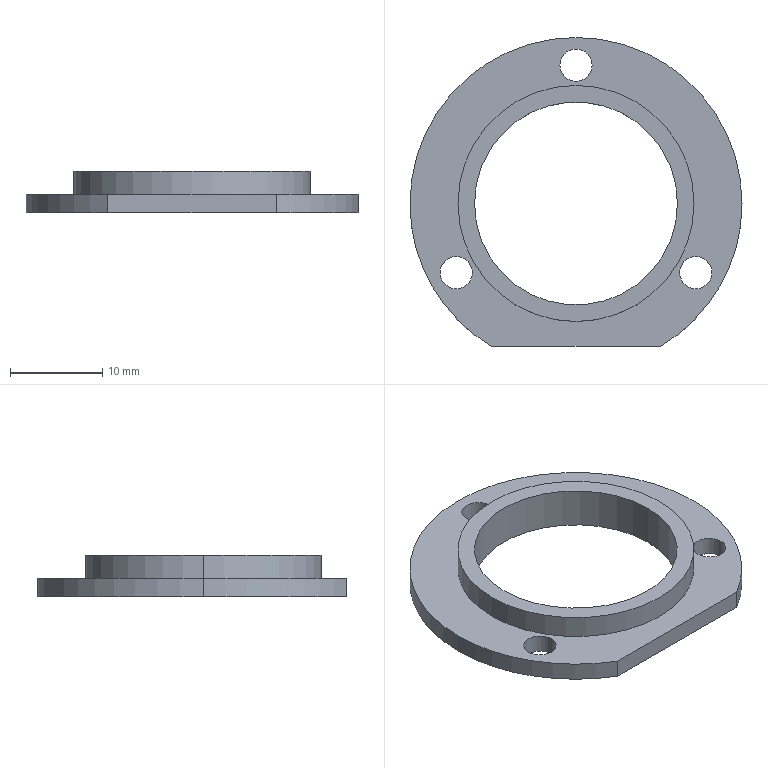Part | SolidWorks | features ICE 3, Extrusion 1 | 1 solid | 17 faces | box 36 x 33.5 x 4.5 mm | volume 1492 mm3 | cylinder 13 | plane 4 | commonest cylinder face diameters 3.5 x6 36 x3 22 x2 25.6 x2
STEP:
#1=CARTESIAN_POINT('',(-14.74,-7.5,2.));
#2=VERTEX_POINT('',#1);
#3=CARTESIAN_POINT('',(-11.24,-7.5,2.));
#4=VERTEX_POINT('',#3);
#5=CARTESIAN_POINT('',(-12.99,-7.5,2.));
#6=DIRECTION('',(0.,0.,1.));
#7=DIRECTION('',(1.,0.,0.));
#8=AXIS2_PLACEMENT_3D('',#5,#6,#7);
#9=CIRCLE('',#8,1.75);
#10=EDGE_CURVE('',#2,#4,#9,.T.);
#11=ORIENTED_EDGE('',*,*,#10,.T.);
#12=CARTESIAN_POINT('',(-11.24,-7.5,0.));
#13=VERTEX_POINT('',#12);
#14=CARTESIAN_POINT('',(-11.24,-7.5,4.5));
#15=DIRECTION('',(0.,0.,-1.));
#16=VECTOR('',#15,1000.);
#17=LINE('',#14,#16);
#18=EDGE_CURVE('',#4,#13,#17,.T.);
#19=ORIENTED_EDGE('',*,*,#18,.T.);
#20=CARTESIAN_POINT('',(-14.74,-7.5,0.));
#21=VERTEX_POINT('',#20);
#22=CARTESIAN_POINT('',(-12.99,-7.5,0.));
#23=DIRECTION('',(0.,0.,-1.));
#24=DIRECTION('',(-1.,0.,0.));
#25=AXIS2_PLACEMENT_3D('',#22,#23,#24);
#26=CIRCLE('',#25,1.75);
#27=EDGE_CURVE('',#13,#21,#26,.T.);
#28=ORIENTED_EDGE('',*,*,#27,.T.);
#29=CARTESIAN_POINT('',(-14.74,-7.5,4.5));
#30=DIRECTION('',(0.,0.,-1.));
#31=VECTOR('',#30,1000.);
#32=LINE('',#29,#31);
#33=EDGE_CURVE('',#2,#21,#32,.T.);
#34=ORIENTED_EDGE('',*,*,#33,.F.);
#35=EDGE_LOOP('',(#11,#19,#28,#34));
#36=FACE_OUTER_BOUND('',#35,.T.);
#37=CARTESIAN_POINT('',(-12.99,-7.5,4.5));
#38=DIRECTION('',(0.,0.,-1.));
#39=DIRECTION('',(-1.,0.,0.));
#40=AXIS2_PLACEMENT_3D('',#37,#38,#39);
#41=CYLINDRICAL_SURFACE('',#40,1.75);
#42=ADVANCED_FACE('',(#36),#41,.F.);
#43=CARTESIAN_POINT('',(11.24,-7.5,2.));
#44=VERTEX_POINT('',#43);
#45=CARTESIAN_POINT('',(14.74,-7.5,2.));
#46=VERTEX_POINT('',#45);
#47=CARTESIAN_POINT('',(12.99,-7.5,2.));
#48=DIRECTION('',(0.,0.,1.));
#49=DIRECTION('',(1.,0.,0.));
#50=AXIS2_PLACEMENT_3D('',#47,#48,#49);
#51=CIRCLE('',#50,1.75);
#52=EDGE_CURVE('',#44,#46,#51,.T.);
#53=ORIENTED_EDGE('',*,*,#52,.T.);
#54=CARTESIAN_POINT('',(14.74,-7.5,0.));
#55=VERTEX_POINT('',#54);
#56=CARTESIAN_POINT('',(14.74,-7.5,4.5));
#57=DIRECTION('',(0.,0.,-1.));
#58=VECTOR('',#57,1000.);
#59=LINE('',#56,#58);
#60=EDGE_CURVE('',#46,#55,#59,.T.);
#61=ORIENTED_EDGE('',*,*,#60,.T.);
#62=CARTESIAN_POINT('',(11.24,-7.5,0.));
#63=VERTEX_POINT('',#62);
#64=CARTESIAN_POINT('',(12.99,-7.5,0.));
#65=DIRECTION('',(0.,0.,-1.));
#66=DIRECTION('',(-1.,0.,0.));
#67=AXIS2_PLACEMENT_3D('',#64,#65,#66);
#68=CIRCLE('',#67,1.75);
#69=EDGE_CURVE('',#55,#63,#68,.T.);
#70=ORIENTED_EDGE('',*,*,#69,.T.);
#71=CARTESIAN_POINT('',(11.24,-7.5,4.5));
#72=DIRECTION('',(0.,0.,-1.));
#73=VECTOR('',#72,1000.);
#74=LINE('',#71,#73);
#75=EDGE_CURVE('',#44,#63,#74,.T.);
#76=ORIENTED_EDGE('',*,*,#75,.F.);
#77=EDGE_LOOP('',(#53,#61,#70,#76));
#78=FACE_OUTER_BOUND('',#77,.T.);
#79=CARTESIAN_POINT('',(12.99,-7.5,4.5));
#80=DIRECTION('',(0.,0.,-1.));
#81=DIRECTION('',(-1.,0.,0.));
#82=AXIS2_PLACEMENT_3D('',#79,#80,#81);
#83=CYLINDRICAL_SURFACE('',#82,1.75);
#84=ADVANCED_FACE('',(#78),#83,.F.);
#85=CARTESIAN_POINT('',(-1.75,15.,2.));
#86=VERTEX_POINT('',#85);
#87=CARTESIAN_POINT('',(1.75,15.,2.));
#88=VERTEX_POINT('',#87);
#89=CARTESIAN_POINT('',(0.,15.,2.));
#90=DIRECTION('',(0.,0.,1.));
#91=DIRECTION('',(1.,0.,0.));
#92=AXIS2_PLACEMENT_3D('',#89,#90,#91);
#93=CIRCLE('',#92,1.75);
#94=EDGE_CURVE('',#86,#88,#93,.T.);
#95=ORIENTED_EDGE('',*,*,#94,.T.);
#96=CARTESIAN_POINT('',(1.75,15.,0.));
#97=VERTEX_POINT('',#96);
#98=CARTESIAN_POINT('',(1.75,15.,4.5));
#99=DIRECTION('',(0.,0.,-1.));
#100=VECTOR('',#99,1000.);
#101=LINE('',#98,#100);
#102=EDGE_CURVE('',#88,#97,#101,.T.);
#103=ORIENTED_EDGE('',*,*,#102,.T.);
#104=CARTESIAN_POINT('',(-1.75,15.,0.));
#105=VERTEX_POINT('',#104);
#106=CARTESIAN_POINT('',(0.,15.,0.));
#107=DIRECTION('',(0.,0.,-1.));
#108=DIRECTION('',(-1.,0.,0.));
#109=AXIS2_PLACEMENT_3D('',#106,#107,#108);
#110=CIRCLE('',#109,1.75);
#111=EDGE_CURVE('',#97,#105,#110,.T.);
#112=ORIENTED_EDGE('',*,*,#111,.T.);
#113=CARTESIAN_POINT('',(-1.75,15.,4.5));
#114=DIRECTION('',(0.,0.,-1.));
#115=VECTOR('',#114,1000.);
#116=LINE('',#113,#115);
#117=EDGE_CURVE('',#86,#105,#116,.T.);
#118=ORIENTED_EDGE('',*,*,#117,.F.);
#119=EDGE_LOOP('',(#95,#103,#112,#118));
#120=FACE_OUTER_BOUND('',#119,.T.);
#121=CARTESIAN_POINT('',(0.,15.,4.5));
#122=DIRECTION('',(0.,0.,-1.));
#123=DIRECTION('',(-1.,0.,0.));
#124=AXIS2_PLACEMENT_3D('',#121,#122,#123);
#125=CYLINDRICAL_SURFACE('',#124,1.75);
#126=ADVANCED_FACE('',(#120),#125,.F.);
#127=CARTESIAN_POINT('',(12.8,0.,2.));
#128=VERTEX_POINT('',#127);
#129=CARTESIAN_POINT('',(-12.8,0.,2.));
#130=VERTEX_POINT('',#129);
#131=CARTESIAN_POINT('',(0.,0.,2.));
#132=DIRECTION('',(0.,0.,1.));
#133=DIRECTION('',(1.,0.,0.));
#134=AXIS2_PLACEMENT_3D('',#131,#132,#133);
#135=CIRCLE('',#134,12.8);
#136=EDGE_CURVE('',#128,#130,#135,.T.);
#137=ORIENTED_EDGE('',*,*,#136,.T.);
#138=CARTESIAN_POINT('',(-12.8,0.,4.5));
#139=VERTEX_POINT('',#138);
#140=CARTESIAN_POINT('',(-12.8,0.,2.));
#141=DIRECTION('',(0.,0.,1.));
#142=VECTOR('',#141,1000.);
#143=LINE('',#140,#142);
#144=EDGE_CURVE('',#130,#139,#143,.T.);
#145=ORIENTED_EDGE('',*,*,#144,.T.);
#146=CARTESIAN_POINT('',(12.8,0.,4.5));
#147=VERTEX_POINT('',#146);
#148=CARTESIAN_POINT('',(0.,0.,4.5));
#149=DIRECTION('',(0.,0.,1.));
#150=DIRECTION('',(1.,0.,0.));
#151=AXIS2_PLACEMENT_3D('',#148,#149,#150);
#152=CIRCLE('',#151,12.8);
#153=EDGE_CURVE('',#147,#139,#152,.T.);
#154=ORIENTED_EDGE('',*,*,#153,.F.);
#155=CARTESIAN_POINT('',(12.8,0.,2.));
#156=DIRECTION('',(0.,0.,1.));
#157=VECTOR('',#156,1000.);
#158=LINE('',#155,#157);
#159=EDGE_CURVE('',#128,#147,#158,.T.);
#160=ORIENTED_EDGE('',*,*,#159,.F.);
#161=EDGE_LOOP('',(#137,#145,#154,#160));
#162=FACE_OUTER_BOUND('',#161,.T.);
#163=CARTESIAN_POINT('',(0.,0.,2.));
#164=DIRECTION('',(0.,0.,1.));
#165=DIRECTION('',(1.,0.,0.));
#166=AXIS2_PLACEMENT_3D('',#163,#164,#165);
#167=CYLINDRICAL_SURFACE('',#166,12.8);
#168=ADVANCED_FACE('',(#162),#167,.T.);
#169=CARTESIAN_POINT('',(-11.,0.,4.5));
#170=VERTEX_POINT('',#169);
#171=CARTESIAN_POINT('',(11.,0.,4.5));
#172=VERTEX_POINT('',#171);
#173=CARTESIAN_POINT('',(0.,0.,4.5));
#174=DIRECTION('',(0.,0.,1.));
#175=DIRECTION('',(1.,0.,0.));
#176=AXIS2_PLACEMENT_3D('',#173,#174,#175);
#177=CIRCLE('',#176,11.);
#178=EDGE_CURVE('',#170,#172,#177,.T.);
#179=ORIENTED_EDGE('',*,*,#178,.T.);
#180=CARTESIAN_POINT('',(11.,0.,0.));
#181=VERTEX_POINT('',#180);
#182=CARTESIAN_POINT('',(11.,0.,4.5));
#183=DIRECTION('',(0.,0.,-1.));
#184=VECTOR('',#183,1000.);
#185=LINE('',#182,#184);
#186=EDGE_CURVE('',#172,#181,#185,.T.);
#187=ORIENTED_EDGE('',*,*,#186,.T.);
#188=CARTESIAN_POINT('',(-11.,0.,0.));
#189=VERTEX_POINT('',#188);
#190=CARTESIAN_POINT('',(0.,0.,0.));
#191=DIRECTION('',(0.,0.,1.));
#192=DIRECTION('',(1.,0.,0.));
#193=AXIS2_PLACEMENT_3D('',#190,#191,#192);
#194=CIRCLE('',#193,11.);
#195=EDGE_CURVE('',#189,#181,#194,.T.);
#196=ORIENTED_EDGE('',*,*,#195,.F.);
#197=CARTESIAN_POINT('',(-11.,0.,4.5));
#198=DIRECTION('',(0.,0.,-1.));
#199=VECTOR('',#198,1000.);
#200=LINE('',#197,#199);
#201=EDGE_CURVE('',#170,#189,#200,.T.);
#202=ORIENTED_EDGE('',*,*,#201,.F.);
#203=EDGE_LOOP('',(#179,#187,#196,#202));
#204=FACE_OUTER_BOUND('',#203,.T.);
#205=CARTESIAN_POINT('',(0.,0.,4.5));
#206=DIRECTION('',(0.,0.,-1.));
#207=DIRECTION('',(-1.,0.,0.));
#208=AXIS2_PLACEMENT_3D('',#205,#206,#207);
#209=CYLINDRICAL_SURFACE('',#208,11.);
#210=ADVANCED_FACE('',(#204),#209,.F.);
#211=CARTESIAN_POINT('',(18.,0.,2.));
#212=VERTEX_POINT('',#211);
#213=CARTESIAN_POINT('',(-18.,0.,2.));
#214=VERTEX_POINT('',#213);
#215=CARTESIAN_POINT('',(0.,0.,2.));
#216=DIRECTION('',(0.,0.,1.));
#217=DIRECTION('',(1.,0.,0.));
#218=AXIS2_PLACEMENT_3D('',#215,#216,#217);
#219=CIRCLE('',#218,18.);
#220=EDGE_CURVE('',#212,#214,#219,.T.);
#221=ORIENTED_EDGE('',*,*,#220,.F.);
#222=CARTESIAN_POINT('',(18.,0.,0.));
#223=VERTEX_POINT('',#222);
#224=CARTESIAN_POINT('',(18.,0.,4.5));
#225=DIRECTION('',(0.,0.,-1.));
#226=VECTOR('',#225,1000.);
#227=LINE('',#224,#226);
#228=EDGE_CURVE('',#212,#223,#227,.T.);
#229=ORIENTED_EDGE('',*,*,#228,.T.);
#230=CARTESIAN_POINT('',(-18.,0.,0.));
#231=VERTEX_POINT('',#230);
#232=CARTESIAN_POINT('',(0.,0.,0.));
#233=DIRECTION('',(0.,0.,1.));
#234=DIRECTION('',(1.,0.,0.));
#235=AXIS2_PLACEMENT_3D('',#232,#233,#234);
#236=CIRCLE('',#235,18.);
#237=EDGE_CURVE('',#223,#231,#236,.T.);
#238=ORIENTED_EDGE('',*,*,#237,.T.);
#239=CARTESIAN_POINT('',(-18.,0.,4.5));
#240=DIRECTION('',(0.,0.,-1.));
#241=VECTOR('',#240,1000.);
#242=LINE('',#239,#241);
#243=EDGE_CURVE('',#214,#231,#242,.T.);
#244=ORIENTED_EDGE('',*,*,#243,.F.);
#245=EDGE_LOOP('',(#221,#229,#238,#244));
#246=FACE_OUTER_BOUND('',#245,.T.);
#247=CARTESIAN_POINT('',(0.,0.,4.5));
#248=DIRECTION('',(0.,0.,-1.));
#249=DIRECTION('',(-1.,0.,0.));
#250=AXIS2_PLACEMENT_3D('',#247,#248,#249);
#251=CYLINDRICAL_SURFACE('',#250,18.);
#252=ADVANCED_FACE('',(#246),#251,.T.);
#253=CARTESIAN_POINT('',(-9.152,-15.5,2.));
#254=VERTEX_POINT('',#253);
#255=CARTESIAN_POINT('',(0.,0.,2.));
#256=DIRECTION('',(0.,0.,1.));
#257=DIRECTION('',(1.,0.,0.));
#258=AXIS2_PLACEMENT_3D('',#255,#256,#257);
#259=CIRCLE('',#258,18.);
#260=EDGE_CURVE('',#214,#254,#259,.T.);
#261=ORIENTED_EDGE('',*,*,#260,.F.);
#262=ORIENTED_EDGE('',*,*,#243,.T.);
#263=CARTESIAN_POINT('',(-9.152,-15.5,0.));
#264=VERTEX_POINT('',#263);
#265=CARTESIAN_POINT('',(0.,0.,0.));
#266=DIRECTION('',(0.,0.,1.));
#267=DIRECTION('',(1.,0.,0.));
#268=AXIS2_PLACEMENT_3D('',#265,#266,#267);
#269=CIRCLE('',#268,18.);
#270=EDGE_CURVE('',#231,#264,#269,.T.);
#271=ORIENTED_EDGE('',*,*,#270,.T.);
#272=CARTESIAN_POINT('',(-9.152,-15.5,4.5));
#273=DIRECTION('',(0.,0.,1.));
#274=VECTOR('',#273,1000.);
#275=LINE('',#272,#274);
#276=EDGE_CURVE('',#264,#254,#275,.T.);
#277=ORIENTED_EDGE('',*,*,#276,.T.);
#278=EDGE_LOOP('',(#261,#262,#271,#277));
#279=FACE_OUTER_BOUND('',#278,.T.);
#280=CARTESIAN_POINT('',(0.,0.,4.5));
#281=DIRECTION('',(0.,0.,-1.));
#282=DIRECTION('',(-1.,0.,0.));
#283=AXIS2_PLACEMENT_3D('',#280,#281,#282);
#284=CYLINDRICAL_SURFACE('',#283,18.);
#285=ADVANCED_FACE('',(#279),#284,.T.);
#286=ORIENTED_EDGE('',*,*,#178,.F.);
#287=CARTESIAN_POINT('',(0.,0.,4.5));
#288=DIRECTION('',(0.,0.,1.));
#289=DIRECTION('',(1.,0.,0.));
#290=AXIS2_PLACEMENT_3D('',#287,#288,#289);
#291=CIRCLE('',#290,11.);
#292=EDGE_CURVE('',#172,#170,#291,.T.);
#293=ORIENTED_EDGE('',*,*,#292,.F.);
#294=EDGE_LOOP('',(#286,#293));
#295=FACE_BOUND('',#294,.T.);
#296=ORIENTED_EDGE('',*,*,#153,.T.);
#297=CARTESIAN_POINT('',(0.,0.,4.5));
#298=DIRECTION('',(0.,0.,1.));
#299=DIRECTION('',(1.,0.,0.));
#300=AXIS2_PLACEMENT_3D('',#297,#298,#299);
#301=CIRCLE('',#300,12.8);
#302=EDGE_CURVE('',#139,#147,#301,.T.);
#303=ORIENTED_EDGE('',*,*,#302,.T.);
#304=EDGE_LOOP('',(#296,#303));
#305=FACE_OUTER_BOUND('',#304,.T.);
#306=CARTESIAN_POINT('',(0.,0.,4.5));
#307=DIRECTION('',(0.,0.,1.));
#308=DIRECTION('',(1.,0.,0.));
#309=AXIS2_PLACEMENT_3D('',#306,#307,#308);
#310=PLANE('',#309);
#311=ADVANCED_FACE('',(#295,#305),#310,.T.);
#312=ORIENTED_EDGE('',*,*,#228,.F.);
#313=CARTESIAN_POINT('',(9.152,-15.5,2.));
#314=VERTEX_POINT('',#313);
#315=CARTESIAN_POINT('',(0.,0.,2.));
#316=DIRECTION('',(0.,0.,1.));
#317=DIRECTION('',(1.,0.,0.));
#318=AXIS2_PLACEMENT_3D('',#315,#316,#317);
#319=CIRCLE('',#318,18.);
#320=EDGE_CURVE('',#314,#212,#319,.T.);
#321=ORIENTED_EDGE('',*,*,#320,.F.);
#322=CARTESIAN_POINT('',(9.152,-15.5,0.));
#323=VERTEX_POINT('',#322);
#324=CARTESIAN_POINT('',(9.152,-15.5,4.5));
#325=DIRECTION('',(0.,0.,-1.));
#326=VECTOR('',#325,1000.);
#327=LINE('',#324,#326);
#328=EDGE_CURVE('',#314,#323,#327,.T.);
#329=ORIENTED_EDGE('',*,*,#328,.T.);
#330=CARTESIAN_POINT('',(0.,0.,0.));
#331=DIRECTION('',(0.,0.,1.));
#332=DIRECTION('',(1.,0.,0.));
#333=AXIS2_PLACEMENT_3D('',#330,#331,#332);
#334=CIRCLE('',#333,18.);
#335=EDGE_CURVE('',#323,#223,#334,.T.);
#336=ORIENTED_EDGE('',*,*,#335,.T.);
#337=EDGE_LOOP('',(#312,#321,#329,#336));
#338=FACE_OUTER_BOUND('',#337,.T.);
#339=CARTESIAN_POINT('',(0.,0.,4.5));
#340=DIRECTION('',(0.,0.,-1.));
#341=DIRECTION('',(-1.,0.,0.));
#342=AXIS2_PLACEMENT_3D('',#339,#340,#341);
#343=CYLINDRICAL_SURFACE('',#342,18.);
#344=ADVANCED_FACE('',(#338),#343,.T.);
#345=CARTESIAN_POINT('',(-12.99,-7.5,0.));
#346=DIRECTION('',(0.,0.,-1.));
#347=DIRECTION('',(-1.,0.,0.));
#348=AXIS2_PLACEMENT_3D('',#345,#346,#347);
#349=CIRCLE('',#348,1.75);
#350=EDGE_CURVE('',#21,#13,#349,.T.);
#351=ORIENTED_EDGE('',*,*,#350,.F.);
#352=ORIENTED_EDGE('',*,*,#27,.F.);
#353=EDGE_LOOP('',(#351,#352));
#354=FACE_BOUND('',#353,.T.);
#355=CARTESIAN_POINT('',(12.99,-7.5,0.));
#356=DIRECTION('',(0.,0.,-1.));
#357=DIRECTION('',(-1.,0.,0.));
#358=AXIS2_PLACEMENT_3D('',#355,#356,#357);
#359=CIRCLE('',#358,1.75);
#360=EDGE_CURVE('',#63,#55,#359,.T.);
#361=ORIENTED_EDGE('',*,*,#360,.F.);
#362=ORIENTED_EDGE('',*,*,#69,.F.);
#363=EDGE_LOOP('',(#361,#362));
#364=FACE_BOUND('',#363,.T.);
#365=CARTESIAN_POINT('',(0.,15.,0.));
#366=DIRECTION('',(0.,0.,-1.));
#367=DIRECTION('',(-1.,0.,0.));
#368=AXIS2_PLACEMENT_3D('',#365,#366,#367);
#369=CIRCLE('',#368,1.75);
#370=EDGE_CURVE('',#105,#97,#369,.T.);
#371=ORIENTED_EDGE('',*,*,#370,.F.);
#372=ORIENTED_EDGE('',*,*,#111,.F.);
#373=EDGE_LOOP('',(#371,#372));
#374=FACE_BOUND('',#373,.T.);
#375=ORIENTED_EDGE('',*,*,#335,.F.);
#376=CARTESIAN_POINT('',(-24.788,-15.5,0.));
#377=DIRECTION('',(-1.,0.,0.));
#378=VECTOR('',#377,1000.);
#379=LINE('',#376,#378);
#380=EDGE_CURVE('',#323,#264,#379,.T.);
#381=ORIENTED_EDGE('',*,*,#380,.T.);
#382=ORIENTED_EDGE('',*,*,#270,.F.);
#383=ORIENTED_EDGE('',*,*,#237,.F.);
#384=EDGE_LOOP('',(#375,#381,#382,#383));
#385=FACE_OUTER_BOUND('',#384,.T.);
#386=ORIENTED_EDGE('',*,*,#195,.T.);
#387=CARTESIAN_POINT('',(0.,0.,0.));
#388=DIRECTION('',(0.,0.,1.));
#389=DIRECTION('',(1.,0.,0.));
#390=AXIS2_PLACEMENT_3D('',#387,#388,#389);
#391=CIRCLE('',#390,11.);
#392=EDGE_CURVE('',#181,#189,#391,.T.);
#393=ORIENTED_EDGE('',*,*,#392,.T.);
#394=EDGE_LOOP('',(#386,#393));
#395=FACE_BOUND('',#394,.T.);
#396=CARTESIAN_POINT('',(0.,0.,0.));
#397=DIRECTION('',(0.,0.,1.));
#398=DIRECTION('',(1.,0.,0.));
#399=AXIS2_PLACEMENT_3D('',#396,#397,#398);
#400=PLANE('',#399);
#401=ADVANCED_FACE('',(#354,#364,#374,#385,#395),#400,.F.);
#402=ORIENTED_EDGE('',*,*,#186,.F.);
#403=ORIENTED_EDGE('',*,*,#292,.T.);
#404=ORIENTED_EDGE('',*,*,#201,.T.);
#405=ORIENTED_EDGE('',*,*,#392,.F.);
#406=EDGE_LOOP('',(#402,#403,#404,#405));
#407=FACE_OUTER_BOUND('',#406,.T.);
#408=CARTESIAN_POINT('',(0.,0.,4.5));
#409=DIRECTION('',(0.,0.,-1.));
#410=DIRECTION('',(-1.,0.,0.));
#411=AXIS2_PLACEMENT_3D('',#408,#409,#410);
#412=CYLINDRICAL_SURFACE('',#411,11.);
#413=ADVANCED_FACE('',(#407),#412,.F.);
#414=ORIENTED_EDGE('',*,*,#10,.F.);
#415=CARTESIAN_POINT('',(-12.99,-7.5,2.));
#416=DIRECTION('',(0.,0.,1.));
#417=DIRECTION('',(1.,0.,0.));
#418=AXIS2_PLACEMENT_3D('',#415,#416,#417);
#419=CIRCLE('',#418,1.75);
#420=EDGE_CURVE('',#4,#2,#419,.T.);
#421=ORIENTED_EDGE('',*,*,#420,.F.);
#422=EDGE_LOOP('',(#414,#421));
#423=FACE_BOUND('',#422,.T.);
#424=ORIENTED_EDGE('',*,*,#52,.F.);
#425=CARTESIAN_POINT('',(12.99,-7.5,2.));
#426=DIRECTION('',(0.,0.,1.));
#427=DIRECTION('',(1.,0.,0.));
#428=AXIS2_PLACEMENT_3D('',#425,#426,#427);
#429=CIRCLE('',#428,1.75);
#430=EDGE_CURVE('',#46,#44,#429,.T.);
#431=ORIENTED_EDGE('',*,*,#430,.F.);
#432=EDGE_LOOP('',(#424,#431));
#433=FACE_BOUND('',#432,.T.);
#434=ORIENTED_EDGE('',*,*,#94,.F.);
#435=CARTESIAN_POINT('',(0.,15.,2.));
#436=DIRECTION('',(0.,0.,1.));
#437=DIRECTION('',(1.,0.,0.));
#438=AXIS2_PLACEMENT_3D('',#435,#436,#437);
#439=CIRCLE('',#438,1.75);
#440=EDGE_CURVE('',#88,#86,#439,.T.);
#441=ORIENTED_EDGE('',*,*,#440,.F.);
#442=EDGE_LOOP('',(#434,#441));
#443=FACE_BOUND('',#442,.T.);
#444=CARTESIAN_POINT('',(0.,-15.5,2.));
#445=DIRECTION('',(-1.,0.,0.));
#446=VECTOR('',#445,1000.);
#447=LINE('',#444,#446);
#448=EDGE_CURVE('',#314,#254,#447,.T.);
#449=ORIENTED_EDGE('',*,*,#448,.F.);
#450=ORIENTED_EDGE('',*,*,#320,.T.);
#451=ORIENTED_EDGE('',*,*,#220,.T.);
#452=ORIENTED_EDGE('',*,*,#260,.T.);
#453=EDGE_LOOP('',(#449,#450,#451,#452));
#454=FACE_OUTER_BOUND('',#453,.T.);
#455=ORIENTED_EDGE('',*,*,#136,.F.);
#456=CARTESIAN_POINT('',(0.,0.,2.));
#457=DIRECTION('',(0.,0.,1.));
#458=DIRECTION('',(1.,0.,0.));
#459=AXIS2_PLACEMENT_3D('',#456,#457,#458);
#460=CIRCLE('',#459,12.8);
#461=EDGE_CURVE('',#130,#128,#460,.T.);
#462=ORIENTED_EDGE('',*,*,#461,.F.);
#463=EDGE_LOOP('',(#455,#462));
#464=FACE_BOUND('',#463,.T.);
#465=CARTESIAN_POINT('',(0.,0.,2.));
#466=DIRECTION('',(0.,0.,1.));
#467=DIRECTION('',(1.,0.,0.));
#468=AXIS2_PLACEMENT_3D('',#465,#466,#467);
#469=PLANE('',#468);
#470=ADVANCED_FACE('',(#423,#433,#443,#454,#464),#469,.T.);
#471=ORIENTED_EDGE('',*,*,#144,.F.);
#472=ORIENTED_EDGE('',*,*,#461,.T.);
#473=ORIENTED_EDGE('',*,*,#159,.T.);
#474=ORIENTED_EDGE('',*,*,#302,.F.);
#475=EDGE_LOOP('',(#471,#472,#473,#474));
#476=FACE_OUTER_BOUND('',#475,.T.);
#477=CARTESIAN_POINT('',(0.,0.,2.));
#478=DIRECTION('',(0.,0.,1.));
#479=DIRECTION('',(1.,0.,0.));
#480=AXIS2_PLACEMENT_3D('',#477,#478,#479);
#481=CYLINDRICAL_SURFACE('',#480,12.8);
#482=ADVANCED_FACE('',(#476),#481,.T.);
#483=ORIENTED_EDGE('',*,*,#448,.T.);
#484=ORIENTED_EDGE('',*,*,#276,.F.);
#485=ORIENTED_EDGE('',*,*,#380,.F.);
#486=ORIENTED_EDGE('',*,*,#328,.F.);
#487=EDGE_LOOP('',(#483,#484,#485,#486));
#488=FACE_OUTER_BOUND('',#487,.T.);
#489=CARTESIAN_POINT('',(-24.788,-15.5,0.));
#490=DIRECTION('',(0.,1.,0.));
#491=DIRECTION('',(0.,0.,1.));
#492=AXIS2_PLACEMENT_3D('',#489,#490,#491);
#493=PLANE('',#492);
#494=ADVANCED_FACE('',(#488),#493,.F.);
#495=ORIENTED_EDGE('',*,*,#102,.F.);
#496=ORIENTED_EDGE('',*,*,#440,.T.);
#497=ORIENTED_EDGE('',*,*,#117,.T.);
#498=ORIENTED_EDGE('',*,*,#370,.T.);
#499=EDGE_LOOP('',(#495,#496,#497,#498));
#500=FACE_OUTER_BOUND('',#499,.T.);
#501=CARTESIAN_POINT('',(0.,15.,4.5));
#502=DIRECTION('',(0.,0.,-1.));
#503=DIRECTION('',(-1.,0.,0.));
#504=AXIS2_PLACEMENT_3D('',#501,#502,#503);
#505=CYLINDRICAL_SURFACE('',#504,1.75);
#506=ADVANCED_FACE('',(#500),#505,.F.);
#507=ORIENTED_EDGE('',*,*,#60,.F.);
#508=ORIENTED_EDGE('',*,*,#430,.T.);
#509=ORIENTED_EDGE('',*,*,#75,.T.);
#510=ORIENTED_EDGE('',*,*,#360,.T.);
#511=EDGE_LOOP('',(#507,#508,#509,#510));
#512=FACE_OUTER_BOUND('',#511,.T.);
#513=CARTESIAN_POINT('',(12.99,-7.5,4.5));
#514=DIRECTION('',(0.,0.,-1.));
#515=DIRECTION('',(-1.,0.,0.));
#516=AXIS2_PLACEMENT_3D('',#513,#514,#515);
#517=CYLINDRICAL_SURFACE('',#516,1.75);
#518=ADVANCED_FACE('',(#512),#517,.F.);
#519=ORIENTED_EDGE('',*,*,#18,.F.);
#520=ORIENTED_EDGE('',*,*,#420,.T.);
#521=ORIENTED_EDGE('',*,*,#33,.T.);
#522=ORIENTED_EDGE('',*,*,#350,.T.);
#523=EDGE_LOOP('',(#519,#520,#521,#522));
#524=FACE_OUTER_BOUND('',#523,.T.);
#525=CARTESIAN_POINT('',(-12.99,-7.5,4.5));
#526=DIRECTION('',(0.,0.,-1.));
#527=DIRECTION('',(-1.,0.,0.));
#528=AXIS2_PLACEMENT_3D('',#525,#526,#527);
#529=CYLINDRICAL_SURFACE('',#528,1.75);
#530=ADVANCED_FACE('',(#524),#529,.F.);
#531=CLOSED_SHELL('',(#42,#84,#126,#168,#210,#252,#285,#311,#344,#401,#413,#470,#482,#494,#506,#518,#530));
#532=MANIFOLD_SOLID_BREP('',#531);
#533=CARTESIAN_POINT('',(0.,0.,0.));
#534=DIRECTION('',(0.,0.,1.));
#535=DIRECTION('',(1.,0.,0.));
#536=AXIS2_PLACEMENT_3D('',#533,#534,#535);
#537=(LENGTH_UNIT()NAMED_UNIT(*)SI_UNIT(.MILLI.,.METRE.));
#538=UNCERTAINTY_MEASURE_WITH_UNIT(LENGTH_MEASURE(0.00001),#537,'','');
#539=(NAMED_UNIT(*)PLANE_ANGLE_UNIT()SI_UNIT($,.RADIAN.));
#540=(NAMED_UNIT(*)SI_UNIT($,.STERADIAN.)SOLID_ANGLE_UNIT());
#541=(GEOMETRIC_REPRESENTATION_CONTEXT(3)GLOBAL_UNCERTAINTY_ASSIGNED_CONTEXT((#538))GLOBAL_UNIT_ASSIGNED_CONTEXT((#537,#539,#540))REPRESENTATION_CONTEXT('',''));
#542=ADVANCED_BREP_SHAPE_REPRESENTATION('',(#532,#536),#541);